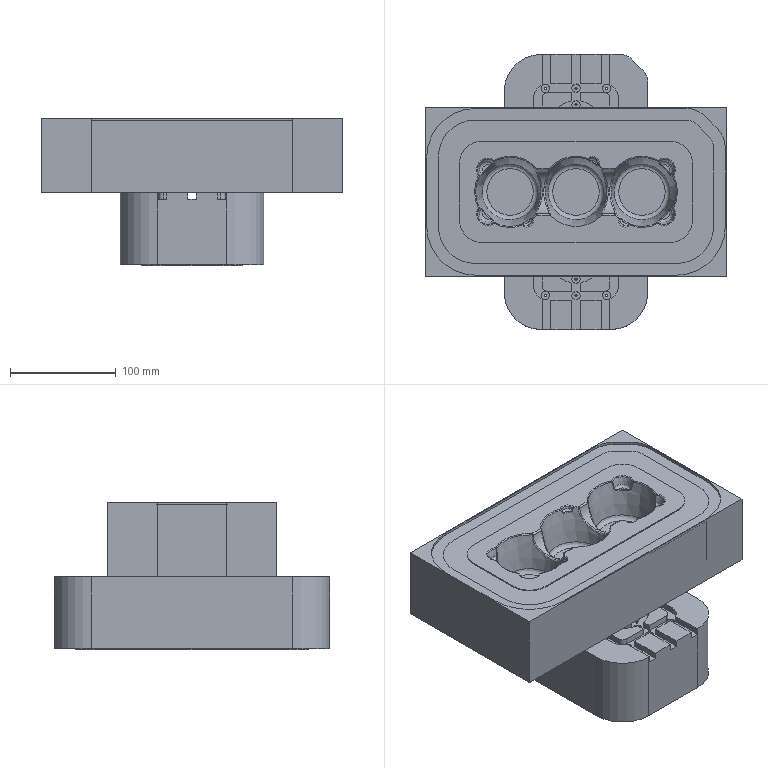NC program | NX | posted with a generic post | part box 284.317 x 260.317 x 139.5 mm
Lines 9197 to 10075 of 226982:
(B5 , TOOL : R2)
N18392 M6
N18394 G53
N18396 G17 G0 G90 X-90.649 Y-47.798 S8000 M3 M8
N18398 G43 Z220.5 H0
N18400 Z72.
N18402 G94 G1 Z69. F4500.
N18404 X-91.341 Y-47.76
N18406 X-91.498 Y-47.743
N18408 X-93.412 Y-47.435
N18410 X-93.627 Y-47.397
N18412 X-94.908 Y-47.053
N18414 X-95.487 Y-46.891
N18416 X-95.835 Y-46.78
N18418 X-96.947 Y-46.36
N18420 X-97.569 Y-46.118
N18422 X-97.691 Y-46.066
N18424 X-97.741 Y-46.044
N18426 X-99.64 Y-45.077
N18428 X-99.812 Y-44.976
N18430 X-101.411 Y-43.938
N18432 X-101.852 Y-43.595
N18434 G2 X-106.218 Y-39.132 R21.375
N18436 G1 X-107.256 Y-37.532
N18438 X-107.355 Y-37.364
N18440 X-108.237 Y-35.635
N18442 X-108.35 Y-35.412
N18444 X-108.398 Y-35.29
N18446 X-108.668 Y-34.596
N18448 X-109.06 Y-33.559
N18450 X-109.171 Y-33.213
N18452 X-109.333 Y-32.634
N18454 X-109.361 Y-32.521
N18456 X-109.549 Y-31.829
N18458 X-109.679 Y-31.342
N18460 X-109.715 Y-31.137
N18462 X-110.024 Y-29.218
N18464 X-110.039 Y-29.061
N18466 X-110.04 Y-29.04
N18468 X-110.079 Y-28.369
N18470 X-110.131 Y-27.331
N18472 X-110.142 Y-26.985
N18474 X-110.149 Y-26.654
N18476 Y26.971
N18478 X-110.131 Y27.328
N18480 X-110.079 Y28.369
N18482 X-110.04 Y29.04
N18484 X-110.024 Y29.218
N18486 X-109.829 Y30.445
N18488 X-109.716 Y31.131
N18490 X-109.679 Y31.342
N18492 X-109.456 Y32.173
N18494 X-109.172 Y33.207
N18496 G2 X-107.257 Y37.531 R21.069
N18498 G1 X-106.219 Y39.131
N18500 X-105.875 Y39.572
N18502 X-104.835 Y40.856
N18504 G2 X-99.812 Y44.975 R21.013
N18506 G1 X-99.645 Y45.074
N18508 X-97.812 Y46.013
N18510 X-97.569 Y46.114
N18512 X-96.876 Y46.387
N18514 X-95.839 Y46.779
N18516 X-95.493 Y46.89
N18518 X-94.914 Y47.052
N18520 X-93.628 Y47.397
N18522 X-93.417 Y47.434
N18524 X-91.497 Y47.743
N18526 X-91.341 Y47.757
N18528 X-90.649 Y47.798
N18530 X-89.265 Y47.868
N18532 X88.919
N18534 X89.265 Y47.861
N18536 X89.607 Y47.85
N18538 X90.649 Y47.798
N18540 X91.32 Y47.759
N18542 X91.498 Y47.743
N18544 X92.723 Y47.548
N18546 X93.627 Y47.397
N18548 X94.453 Y47.175
N18550 X95.487 Y46.891
N18552 G2 X99.812 Y44.976 R21.076
N18554 G1 X101.411 Y43.938
N18556 X101.852 Y43.595
N18558 X102.759 Y42.86
N18560 X103.136 Y42.554
N18562 X103.582 Y42.125 Z68.999
N18564 X104.618 Y41.083
N18566 X104.862 Y40.824 Z69.
N18568 X105.98 Y39.44
N18570 X106.218 Y39.132
N18572 X107.256 Y37.532
N18574 X107.355 Y37.364
N18576 X108.294 Y35.532
N18578 X108.395 Y35.289
N18580 X108.526 Y34.96
N18582 X109.06 Y33.559
N18584 X109.171 Y33.213
N18586 X109.333 Y32.634
N18588 X109.361 Y32.521
N18590 X109.456 Y32.175
N18592 X109.679 Y31.342
N18594 X109.715 Y31.137
N18596 X109.829 Y30.445
N18598 X110.024 Y29.218
N18600 X110.039 Y29.061
N18602 X110.079 Y28.369
N18604 X110.149 Y26.985
N18606 Y-26.639
N18608 X110.142 Y-26.985
N18610 X110.131 Y-27.328
N18612 X110.079 Y-28.369
N18614 X110.04 Y-29.04
N18616 X110.024 Y-29.218
N18618 X109.716 Y-31.131
N18620 X109.679 Y-31.342
N18622 X109.334 Y-32.628
N18624 X109.172 Y-33.207
N18626 X109.061 Y-33.554
N18628 X108.667 Y-34.597
N18630 X108.396 Y-35.286
N18632 X108.294 Y-35.532
N18634 X107.358 Y-37.359
N18636 X107.257 Y-37.531
N18638 X106.219 Y-39.131
N18640 X105.875 Y-39.572
N18642 X105.171 Y-40.442
N18644 X104.952 Y-40.713 Z68.998
N18646 X104.862 Y-40.824 Z69.
N18648 G2 X99.812 Y-44.975 R21.229
N18650 G1 X99.645 Y-45.074
N18652 X97.812 Y-46.013
N18654 X97.569 Y-46.114
N18656 X97.24 Y-46.245
N18658 X95.839 Y-46.779
N18660 X95.493 Y-46.89
N18662 X94.914 Y-47.052
N18664 X93.627 Y-47.397
N18666 X92.725 Y-47.548
N18668 X91.497 Y-47.743
N18670 X91.341 Y-47.757
N18672 X90.649 Y-47.798
N18674 X89.611 Y-47.85
N18676 X89.265 Y-47.861
N18678 X88.934 Y-47.868
N18680 X-89.251
N18682 X-89.607 Y-47.85
N18684 X-90.649 Y-47.798
N18686 Y-47.743
N18688 Y-47.512
N18690 X-91.373 Y-47.468
N18692 X-91.671 Y-47.427
N18694 X-93.071 Y-47.201
N18696 X-93.468 Y-47.136
N18698 X-93.757 Y-47.067
N18700 X-94.455 Y-46.879
N18702 G2 X-97.641 Y-45.775 R20.417
N18704 X-109.253 Y-31.829 R20.708
N18706 G1 X-109.346 Y-31.483
N18708 X-109.416 Y-31.187
N18710 X-109.708 Y-29.392
N18712 X-109.748 Y-29.093
N18714 X-109.751 Y-29.061
N18716 X-109.821 Y-27.82
N18718 X-109.854 Y-27.161
N18720 X-109.86 Y-26.985
N18722 X-109.863 Y26.801
N18724 X-109.846 Y27.331
N18726 G2 X-108.735 Y33.611 R20.049
N18728 G1 X-108.295 Y34.767
N18730 X-108.181 Y35.057
N18732 X-108.056 Y35.364
N18734 G2 X-102.685 Y42.554 R20.975
N18736 G1 X-102.524 Y42.684
N18738 X-101.721 Y43.334
N18740 X-101.316 Y43.651
N18742 G2 X-95.493 Y46.588 R20.765
N18744 G1 X-95.168 Y46.685
N18746 X-94.825 Y46.78
N18748 X-94.692 Y46.815
N18750 X-93.763 Y47.066
N18752 X-93.468 Y47.136
N18754 X-93.306 Y47.163
N18756 G2 X-88.919 Y47.583 R20.239
N18758 G1 X89.265 Y47.579
N18760 X91.084 Y47.487
N18762 X91.341 Y47.47
N18764 X91.373 Y47.467
N18766 X91.671 Y47.427
N18768 X93.468 Y47.135
N18770 X93.757 Y47.067
N18772 X94.801 Y46.786
N18774 G2 X104.835 Y40.405 R20.401
N18776 X107.107 Y37.215 R21.444
N18778 X108.754 Y33.559 R19.283
N18780 G1 X108.898 Y33.124
N18782 G2 X109.748 Y29.093 R20.718
N18784 G1 X109.751 Y29.061
N18786 X109.821 Y27.82
N18788 X109.854 Y27.161
N18790 X109.86 Y26.985
N18792 X109.863 Y-26.801
N18794 X109.846 Y-27.331
N18796 G2 X108.18 Y-35.057 R20.332
N18798 G1 X108.056 Y-35.364
N18800 G2 X105.615 Y-39.44 R19.949
N18802 G1 X104.835 Y-40.404
N18804 X104.773 Y-40.478
N18806 G2 X95.168 Y-46.685 R20.616
N18808 G1 X94.825 Y-46.78
N18810 X93.763 Y-47.066
N18812 X93.468 Y-47.135
N18814 X92.892 Y-47.231
N18816 G2 X89.435 Y-47.573 R18.487
N18818 G1 X88.919 Y-47.583
N18820 X-89.265 Y-47.579
N18822 X-90.649 Y-47.512
N18824 Y-47.226
N18826 G2 X-97.569 Y-45.49 R19.767
N18828 X-109.575 Y-26.985 R20.392
N18830 G1 X-109.578 Y26.74
N18832 X-109.575 Y26.985
N18834 G2 X-105.514 Y39.106 R20.649
N18836 X-93.238 Y46.884 R20.415
N18838 X-88.919 Y47.298 R20.666
N18840 G1 X89.265 Y47.294
N18842 X90.995 Y47.206
N18844 G2 X97.201 Y45.646 R19.84
N18846 X109.575 Y26.985 R20.388
N18848 G1 X109.578 Y-26.74
N18850 X109.575 Y-26.985
N18852 G2 X105.515 Y-39.106 R20.608
N18854 X88.919 Y-47.298 R20.491
N18856 G1 X-89.265 Y-47.294
N18858 X-90.649 Y-47.226
N18860 X-90.634 Y-46.942
N18862 X-91.198 Y-46.908
N18864 G2 X-96.877 Y-45.469 R20.309
N18866 G1 X-97.255 Y-45.322
N18868 G2 X-101.555 Y-42.735 R19.15
N18870 X-109.275 Y-27.331 R19.997
N18872 G1 X-109.292 Y-26.985
N18874 X-109.293 Y-26.946
N18876 X-109.29 Y27.028
N18878 G2 X-106.745 Y36.673 R19.973
N18880 X-89.265 Y47.01 R20.094
N18882 G1 X89.265
N18884 G2 X107.389 Y35.422 R20.108
N18886 G1 X107.456 Y35.289
N18888 G2 X109.293 Y26.946 R20.37
N18890 G1 X109.29 Y-27.028
N18892 G2 X106.745 Y-36.673 R19.973
N18894 X91.135 Y-46.912 R20.082
N18896 G1 X89.265 Y-47.01
N18898 X-89.265
N18900 X-90.634 Y-46.942
N18902 X-90.602 Y-46.658
N18904 G2 X-93.341 Y-46.284 R19.257
N18906 X-100.748 Y-43.004 R20.19
N18908 X-108.349 Y-31.898 R19.674
N18910 X-109.006 Y-27.009 R19.531
N18912 G1 X-109.008 Y26.961
N18914 G2 X-104.794 Y39.094 R19.862
N18916 X-89.268 Y46.726 R19.837
N18918 G1 X89.262
N18920 G2 X93.341 Y46.283 R20.044
N18922 X101.156 Y42.69 R19.954
N18924 X108.349 Y31.898 R19.619
N18926 X109.006 Y27.009 R19.487
N18928 G1 X109.008 Y-26.961
N18930 G2 X104.143 Y-39.895 R19.977
N18932 X89.268 Y-46.726 R19.927
N18934 G1 X-89.262
N18936 X-90.602 Y-46.658
N18938 X-90.587 Y-46.373
N18940 X-90.647 Y-46.37
N18942 X-90.987 Y-46.351
N18944 X-91.308 Y-46.326
N18946 G2 X-108.72 Y-26.985 R19.549
N18948 G1 X-108.722 Y26.904
N18950 G2 X-89.183 Y46.441 R19.568
N18952 G1 X89.265 Y46.439
N18954 G2 X108.602 Y29.061 R19.542
N18956 G1 X108.606 Y29.027
N18958 X108.631 Y28.715
N18960 X108.65 Y28.382
N18962 X108.72 Y26.985
N18964 X108.722 Y-26.904
N18966 X108.631 Y-28.715
N18968 X108.601 Y-29.061
N18970 X108.596 Y-29.106
N18972 G2 X89.183 Y-46.441 R19.566
N18974 G1 X-89.265 Y-46.439
N18976 X-90.587 Y-46.373
N18978 X-90.572 Y-46.088
N18980 X-91.043 Y-46.061
N18982 G2 X-108.434 Y-26.985 R19.275
N18984 G1 X-108.438 Y-21.936
N18986 X-108.437 Y26.843
N18988 G2 X-108.319 Y29.036 R44.188
N18990 X-94.344 Y45.432 R19.241
N18992 X-89.265 Y46.153 R18.273
N18994 G1 X-87.387 Y46.158
N18996 X89.062 Y46.157
N18998 X89.265 Y46.153
N19000 G2 X93.416 Y45.681 R18.878
N19002 X108.295 Y29.198 R19.259
N19004 G1 X108.311 Y29.084
N19006 X108.314 Y29.061
N19008 X108.341 Y28.767
N19010 X108.434 Y26.985
N19012 X108.438 Y21.936
N19014 X108.437 Y-26.843
N19016 G2 X108.319 Y-29.037 R43.992
N19018 X89.265 Y-46.153 R19.291
N19020 G1 X87.535 Y-46.158
N19022 X-89.062 Y-46.157
N19024 X-89.265 Y-46.153
N19026 X-89.4 Y-46.148
N19028 X-90.572 Y-46.088
N19030 X-90.557 Y-45.804
N19032 G2 X-108.153 Y-26.639 R18.972
N19034 G1 Y26.781
N19036 G2 X-89.265 Y45.868 R18.996
N19038 G1 X-87.531 Y45.873
N19040 X89.123 Y45.871
N19042 X89.265 Y45.868
N19044 G2 X108.153 Y26.639 R18.98
N19046 G1 Y-26.781
N19048 G2 X89.265 Y-45.868 R18.996
N19050 G1 X87.531 Y-45.873
N19052 X-89.123 Y-45.871
N19054 X-89.265 Y-45.868
N19056 X-89.458 Y-45.86
N19058 X-90.445 Y-45.81
N19060 X-90.557 Y-45.804
N19062 X-90.542 Y-45.519
N19064 G2 X-107.802 Y-28.223 R18.626
N19066 G1 X-107.866 Y-26.903
N19068 X-107.868 Y26.72
N19070 G2 X-89. Y45.587 R18.721
N19072 G1 X-88.919 Y45.588
N19074 X89.183 Y45.585
N19076 G2 X106.994 Y32.521 R18.729
N19078 X107.866 Y26.903 R18.927
N19080 G1 X107.868 Y-26.72
N19082 G2 X88.919 Y-45.588 R18.73
N19084 G1 X-89.183 Y-45.585
N19086 X-90.542 Y-45.519
N19088 X-90.527 Y-45.234
N19090 G2 X-107.494 Y-28.607 R18.362
N19092 G1 X-107.581 Y-26.964
N19094 X-107.583 Y26.639
N19096 G2 X-90.995 Y45.205 R18.433
N19098 G1 X-90.383 Y45.242
N19100 X-89.289 Y45.298
N19102 X-89.265 Y45.299
N19104 X89.265
N19106 G2 X106.446 Y33.213 R18.387
N19108 X107.581 Y26.964 R17.928
N19110 G1 X107.583 Y-26.639
N19112 G2 X89.265 Y-45.299 R18.435
N19114 G1 X-89.265
N19116 X-90.527 Y-45.234
N19118 X-90.513 Y-44.95
N19120 G2 X-107.294 Y-26.985 R18.091
N19122 G1 X-107.298 Y-18.573
N19124 X-107.294 Y26.985
N19126 G2 X-106.094 Y33.338 R18.163
N19128 X-89.265 Y45.014 R18.132
N19130 G1 X89.263
N19132 G2 X103.964 Y37.364 R18.152
N19134 X107.294 Y26.985 R18.404
N19136 G1 X107.298 Y18.573
N19138 X107.294 Y-26.985
N19140 G2 X106.305 Y-32.781 R18.457
N19142 X89.265 Y-45.014 R18.164
N19144 G1 X-89.263
N19146 X-90.513 Y-44.95
N19148 X-90.498 Y-44.665
N19150 G2 X-107.005 Y-27.08 R17.788
N19152 G1 X-107.008 Y-26.985
N19154 X-107.012 Y-26.741
N19156 X-107.013 Y-26.639
N19158 X-107.011 Y26.885
N19160 G2 X-89.165 Y44.73 R17.87
N19162 G1 X89.021 Y44.731
N19164 G2 X93.07 Y44.295 R19.93
N19166 X107.005 Y27.08 R17.829
N19168 G1 X107.008 Y26.985
N19170 X107.012 Y26.741
N19172 X107.013 Y26.639
N19174 X107.011 Y-26.885
N19176 G2 X89.165 Y-44.73 R17.87
N19178 G1 X-89.021 Y-44.731
N19180 X-89.265 Y-44.727
N19182 X-89.359 Y-44.724
N19184 X-89.611 Y-44.711
N19186 X-90.498 Y-44.665
N19188 X-90.482 Y-44.38
N19190 G2 X-106.716 Y-27.137 R17.508
N19192 G1 X-106.722 Y-26.985
N19194 X-106.728 Y-26.457
N19196 X-106.726 Y26.824
N19198 G2 X-104.664 Y35.113 R17.493
N19200 X-89.462 Y44.433 R17.525
N19202 G1 X-88.919 Y44.447
N19204 X89.081 Y44.445
N19206 G2 X103.176 Y37.466 R17.595
N19208 X106.722 Y26.985 R17.748
N19210 G1 X106.728 Y26.457
N19212 X106.726 Y-26.824
N19214 G2 X89.265 Y-44.441 R17.584
N19216 G1 X88.755 Y-44.447
N19218 X-89.081 Y-44.445
N19220 X-89.265 Y-44.441
N19222 X-89.417 Y-44.435
N19224 X-90.303 Y-44.39
N19226 X-90.482 Y-44.38
N19228 X-90.461 Y-44.095
N19230 G2 X-106.436 Y-26.985 R17.248
N19232 G1 X-106.443 Y-26.518
N19234 X-106.441 Y26.763
N19236 G2 X-88.919 Y44.162 R17.312
N19238 G1 X89.14 Y44.158
N19240 G2 X94.773 Y43.218 R17.668
N19242 X106.436 Y26.985 R17.273
N19244 G1 X106.443 Y26.518
N19246 X106.441 Y-26.763
N19248 G2 X88.919 Y-44.162 R17.312
N19250 G1 X-89.14 Y-44.158
N19252 X-89.803 Y-44.13
N19254 X-90.461 Y-44.095
N19256 X-90.446 Y-43.811
N19258 G2 X-106.154 Y-26.921 R16.957
N19260 G1 X-106.157 Y26.701
N19262 G2 X-88.634 Y43.877 R17.043
N19264 G1 X89.201 Y43.873
N19266 G2 X105.941 Y29.482 R16.96
N19268 G1 X106.032 Y28.875
N19270 X106.05 Y28.715
N19272 X106.065 Y28.562
N19274 X106.099 Y28.023
N19276 X106.154 Y26.921
N19278 X106.157 Y-26.701
N19280 G2 X88.634 Y-43.877 R17.042
N19282 G1 X-89.201 Y-43.873
N19284 X-90.446 Y-43.811
N19286 X-90.431 Y-43.526
N19288 G2 X-105.424 Y-30.689 R16.629
N19290 X-105.873 Y-26.64 R17.53
N19292 G1 X-105.872 Y26.639
N19294 G2 X-90.649 Y43.514 R16.731
N19296 G1 X-90.365 Y43.53
N19298 X-89.27 Y43.587
N19300 X-88.985 Y43.592
N19302 X-88.919
N19304 X88.919
N19306 G2 X104.143 Y34.256 R16.721
N19308 X105.814 Y28.023 R16.056
N19310 G1 X105.868 Y26.985
N19312 X105.873 Y26.64
N19314 X105.872 Y-26.639
N19316 G2 X90.649 Y-43.514 R16.729
N19318 G1 X90.365 Y-43.53
N19320 X89.27 Y-43.587
N19322 X88.985 Y-43.592
N19324 X88.919
N19326 X-88.919
N19328 X-89.261 Y-43.587
N19330 X-90.431 Y-43.526
N19332 X-90.415 Y-43.241
N19334 X-90.633 Y-43.229
N19336 G2 X-105.587 Y-26.701 R16.403
N19338 G1 X-105.588 Y-26.355
N19340 X-105.587 Y26.579
N19342 G2 X-88.858 Y43.307 R16.464
N19344 G1 X88.919
N19346 G2 X92.764 Y42.9 R17.06
N19348 X105.587 Y26.701 R16.405
N19350 G1 X105.588 Y26.355
N19352 X105.587 Y-26.579
N19354 G2 X88.858 Y-43.307 R16.467
N19356 G1 X-88.919
N19358 X-89.264 Y-43.302
N19360 X-89.955 Y-43.266
N19362 X-90.415 Y-43.241
N19364 X-90.4 Y-42.956
N19366 G2 X-104.489 Y-31.921 R16.067
N19368 X-105.303 Y-26.416 R17.107
N19370 G1 X-105.299 Y26.867
N19372 G2 X-89.147 Y43.018 R16.167
N19374 G1 X-83.254 Y43.022
N19376 X89.039 Y43.02
N19378 G2 X95.955 Y41.516 R16.73
N19380 X105.296 Y26.985 R16.104
N19382 G1 X105.303 Y26.416
N19384 X105.299 Y-26.867
N19386 G2 X89.147 Y-43.018 R16.166
N19388 G1 X83.254 Y-43.022
N19390 X-89.039 Y-43.02
N19392 X-89.265 Y-43.015
N19394 X-89.376 Y-43.01
N19396 X-90.303 Y-42.962
N19398 X-90.4 Y-42.956
N19400 X-90.384 Y-42.671
N19402 G2 X-105.002 Y-27.153 R15.804
N19404 G1 X-105.016 Y-26.639
N19406 Y26.639
N19408 G2 X-104.857 Y29.039 R17.293
N19410 X-89.265 Y42.728 R15.86
N19412 G1 X-88.573 Y42.737
N19414 X88.919 Y42.735
N19416 G2 X104.894 Y28.782 R15.849
N19418 X105.016 Y26.639 R20.313
N19420 G1 Y-26.639
N19422 G2 X103.797 Y-32.949 R16.109
N19424 X89.265 Y-42.728 R15.869
N19426 G1 X88.573 Y-42.737
N19428 X-88.919 Y-42.735
N19430 X-89.432 Y-42.721
N19432 X-90.384 Y-42.671
N19434 X-90.366 Y-42.386
N19436 G2 X-104.68 Y-27.869 R15.479
N19438 G1 X-104.728 Y-26.879
N19440 X-104.733 Y-26.293
N19442 X-104.73 Y26.744
N19444 G2 X-103.374 Y33.213 R15.519
N19446 X-89.265 Y42.443 R15.572
N19448 G1 X-88.675 Y42.452
N19450 X88.919 Y42.45
N19452 G2 X102.477 Y34.943 R15.627
N19454 X104.732 Y26.639 R15.801
N19456 G1 X104.73 Y-26.744
N19458 G2 X102.973 Y-34.037 R15.504
N19460 X89.265 Y-42.443 R15.567
N19462 G1 X88.675 Y-42.452
N19464 X-88.919 Y-42.45
N19466 X-89.49 Y-42.433
N19468 X-90.366 Y-42.386
N19470 X-90.35 Y-42.102
N19472 G2 X-104.372 Y-28.253 R15.215
N19474 G1 X-104.442 Y-26.939
N19476 X-104.448 Y-26.599
N19478 X-104.446 Y26.682
N19480 G2 X-88.614 Y42.167 R15.345
N19482 G1 X88.878
N19484 G2 X100.478 Y37.161 R15.381
N19486 X104.448 Y26.599 R15.432
N19488 G1 X104.446 Y-26.682
N19490 G2 X88.614 Y-42.167 R15.345
N19492 G1 X-88.878
N19494 X-89.218 Y-42.161
N19496 X-89.265 Y-42.159
N19498 X-90.35 Y-42.102
N19500 X-90.332 Y-41.818
N19502 G2 X-104.155 Y-27.001 R14.971
N19504 G1 X-104.163 Y-26.639
N19506 X-104.162 Y26.618
N19508 G2 X-92.361 Y41.534 R15.058
N19510 X-88.922 Y41.882 R16.461
N19512 G1 X88.916
N19514 G2 X102.861 Y32.981 R15.014
N19516 X104.163 Y26.639 R15.632
N19518 G1 X104.162 Y-26.618
N19520 G2 X90.649 Y-41.798 R15.04
N19522 G1 X90.348 Y-41.818
N19524 X89.267 Y-41.875
N19526 X88.922 Y-41.882
N19528 X-88.916
N19530 X-89.263 Y-41.875
N19532 X-90.263 Y-41.822
N19534 X-90.332 Y-41.818
N19536 X-90.301 Y-41.534
N19538 G2 X-103.869 Y-26.985 R14.664
N19540 G1 X-103.878 Y-26.375
N19542 X-103.876 Y26.639
N19544 G2 X-92.293 Y41.256 R14.773
N19546 X-88.838 Y41.597 R16.102
N19548 G1 X88.998 Y41.595
N19550 G2 X101.825 Y34.371 R14.776
N19552 X103.878 Y26.375 R15.062
N19554 G1 X103.876 Y-26.639
N19556 G2 X88.838 Y-41.597 R14.77
N19558 G1 X-88.998 Y-41.595
N19560 X-89.265 Y-41.589
N19562 X-89.314 Y-41.587
N19564 X-90.301 Y-41.534
N19566 X-90.285 Y-41.249
N19568 G2 X-103.582 Y-26.985 R14.379
N19570 G1 X-103.593 Y-26.293
N19572 X-103.59 Y26.639
N19574 G2 X-89.265 Y41.301 R14.466
N19576 G1 X-88.573 Y41.312
N19578 X88.919 Y41.31
N19580 G2 X94.556 Y40.249 R14.802
N19582 X103.582 Y26.985 R14.365
N19584 G1 X103.593 Y26.293
N19586 X103.59 Y-26.639
N19588 G2 X89.265 Y-41.301 R14.466
N19590 G1 X88.573 Y-41.312
N19592 X-88.919 Y-41.31
N19594 X-89.611 Y-41.285
N19596 X-89.957 Y-41.267
N19598 X-90.285 Y-41.249
N19600 X-90.268 Y-40.963
N19602 G2 X-103.016 Y-29.665 R14.057
N19604 X-103.308 Y-26.293 R15.915
N19606 G1 X-103.305 Y26.639
N19608 G2 X-89.265 Y41.016 R14.18
N19610 G1 X-88.573 Y41.027
N19612 X88.919 Y41.025
N19614 G2 X100.438 Y35.411 R14.202
N19616 X103.302 Y26.837 R14.342
N19618 G1 X103.308 Y26.293
N19620 X103.305 Y-26.639
N19622 G2 X89.265 Y-41.016 R14.177
N19624 G1 X88.573 Y-41.027
N19626 X-88.919 Y-41.025
N19628 X-89.611 Y-41.
N19630 X-90.106 Y-40.973
N19632 X-90.268 Y-40.963
N19634 X-90.25 Y-40.679
N19636 G2 X-103.001 Y-27.228 R13.799
N19638 G1 X-103.021 Y-26.639
N19640 X-103.02 Y26.725
N19642 G2 X-101.952 Y32.175 R13.917
N19644 X-89.265 Y40.732 R13.879
N19646 G1 X-88.655 Y40.742
N19648 X88.919 Y40.74
N19650 G2 X93.622 Y39.991 R14.393
N19652 X103.016 Y26.897 R13.825
N19654 G1 X103.021 Y26.639
N19656 X103.022 Y26.557
N19658 X103.02 Y-26.725
N19660 G2 X102.413 Y-30.899 R14.116
N19662 X89.265 Y-40.732 R13.881
N19664 G1 X88.655 Y-40.742
N19666 X-88.919 Y-40.74
N19668 X-89.507 Y-40.72
N19670 X-90.164 Y-40.685
N19672 X-90.25 Y-40.679
N19674 X-90.221 Y-40.396
N19676 G2 X-102.73 Y-26.956 R13.526
N19678 G1 X-102.738 Y-26.618
N19680 X-102.736 Y26.639
N19682 G2 X-92.017 Y40.148 R13.641
N19684 X-88.941 Y40.456 R15.94
N19686 G1 X88.897
N19688 G2 X97.25 Y37.78 R13.882
N19690 X102.73 Y26.956 R13.625
N19692 G1 X102.738 Y26.618
N19694 X102.736 Y-26.639
N19696 G2 X90.395 Y-40.386 R13.617
N19698 G1 X90.303 Y-40.392
N19700 X89.265 Y-40.447
N19702 X88.941 Y-40.456
N19704 X-88.897
N19706 X-89.236 Y-40.449
N19708 X-89.265 Y-40.447
N19710 X-90.221 Y-40.396
N19712 X-90.205 Y-40.111
N19714 G2 X-102.442 Y-27.015 R13.268
N19716 G1 X-102.451 Y-26.682
N19718 X-102.452 Y-26.639
N19720 X-102.451 Y26.598
N19722 G2 X-101.74 Y31.133 R13.818
N19724 X-88.922 Y40.172 R13.343
N19726 G1 X88.917 Y40.171
N19728 G2 X99.064 Y35.746 R13.411
N19730 X102.442 Y27.015 R13.445
N19732 G1 X102.451 Y26.682
N19734 X102.452 Y26.639
N19736 X102.451 Y-26.598
N19738 G2 X101.741 Y-31.132 R13.847
N19740 X88.922 Y-40.172 R13.345
N19742 G1 X-88.917 Y-40.171
N19744 X-89.265 Y-40.162
N19746 X-90.205 Y-40.111
N19748 X-90.189 Y-39.826
N19750 G2 X-102.156 Y-26.985 R12.954
N19752 G1 X-102.167 Y-26.293
N19754 X-102.164 Y26.639
N19756 G2 X-100.855 Y32.521 R13.043
N19758 X-89.173 Y39.879 R13.019
N19760 G1 X-88.573 Y39.887
N19762 X89.016 Y39.883
N19764 G2 X94.455 Y38.75 R13.358
N19766 X102.156 Y26.985 R12.974
N19768 G1 X102.167 Y26.293
N19770 X102.164 Y-26.639
N19772 G2 X101.023 Y-32.175 R13.368
N19774 X89.173 Y-39.879 R13.045
N19776 G1 X88.573 Y-39.887
N19778 X-89.016 Y-39.883
N19780 X-89.611 Y-39.858
N19782 X-89.956 Y-39.839
N19784 X-90.189 Y-39.826
N19786 X-90.17 Y-39.54
N19788 G2 X-101.87 Y-26.985 R12.661
N19790 G1 X-101.882 Y-26.293
N19792 X-101.879 Y26.639
N19794 G2 X-89.11 Y39.595 R12.772
N19796 G1 X-88.573 Y39.602
N19798 X88.919 Y39.599
N19800 G2 X100.706 Y32.198 R12.757
N19802 X101.87 Y26.985 R12.922
N19804 G1 X101.882 Y26.293
N19806 X101.879 Y-26.639
N19808 G2 X89.11 Y-39.595 R12.772
N19810 G1 X88.573 Y-39.602
N19812 X-88.919 Y-39.599
N19814 X-89.408 Y-39.583
N19816 X-90.17 Y-39.54
N19818 X-90.121 Y-39.258
N19820 G2 X-101.591 Y-26.856 R12.401
N19822 G1 X-101.596 Y-26.639
N19824 X-101.597 Y-26.516
N19826 X-101.595 Y26.639
N19828 G2 X-90.303 Y39.247 R12.477
N19830 G1 X-90.139 Y39.259
N19832 X-89.047 Y39.313
N19834 X-83.15 Y39.316
N19836 X88.919 Y39.315
N19838 G2 X95.619 Y37.498 R12.759
N19840 X101.596 Y26.639 R12.494
N19842 G1 X101.597 Y26.516
N19844 X101.595 Y-26.639
N19846 G2 X90.303 Y-39.247 R12.475
N19848 G1 X90.138 Y-39.259
N19850 X89.047 Y-39.313
N19852 X83.15 Y-39.316
N19854 X-88.919 Y-39.315
N19856 X-89.466 Y-39.295
N19858 X-89.794 Y-39.277
N19860 X-90.121 Y-39.258
N19862 X-90.104 Y-38.974
N19864 G2 X-101.304 Y-26.915 R12.123
N19866 G1 X-101.311 Y-26.639
N19868 X-101.312 Y-26.577
N19870 X-101.309 Y26.705
N19872 G2 X-100.153 Y32.013 R12.39
N19874 X-90.303 Y38.961 R12.172
N19876 X-88.919 Y39.03 R28.075
N19878 G1 X88.919
N19880 G2 X93.302 Y38.287 R12.711
N19882 X101.304 Y26.915 R12.121
N19884 G1 X101.311 Y26.639
N19886 X101.312 Y26.577
N19888 X101.309 Y-26.705
N19890 G2 X100.421 Y-31.398 R12.52
N19892 X90.303 Y-38.961 R12.184
N19894 X88.919 Y-39.03 R28.235
N19896 G1 X-88.919
N19898 X-89.523 Y-39.007
N19900 X-89.852 Y-38.989
N19902 X-90.104 Y-38.974
N19904 X-90.086 Y-38.689
N19906 G2 X-101.016 Y-26.985 R11.816
N19908 G1 X-101.027 Y-26.639
N19910 X-101.026 Y26.639
N19912 G2 X-100.462 Y30.445 R12.478
N19914 X-90.303 Y38.676 R11.909
N19916 G1 X-90.01 Y38.695
N19918 X-89.279 Y38.734
N19920 X-88.921 Y38.746
N19922 X88.917
N19924 G2 X100.085 Y31.483 R11.907
N19926 X101.027 Y26.639 R12.303
N19928 G1 X101.026 Y-26.639
N19930 G2 X90.303 Y-38.676 R11.922
N19932 G1 X90.01 Y-38.695
N19934 X89.279 Y-38.735
N19936 X88.921 Y-38.746
N19938 X-88.917
N19940 X-89.253 Y-38.736
N19942 X-89.909 Y-38.7
N19944 X-90.086 Y-38.689
N19946 X-90.069 Y-38.405
N19948 G2 X-100.728 Y-27.035 R11.529
N19950 G1 X-100.74 Y-26.699
N19952 X-100.741 Y26.581
N19954 G2 X-88.92 Y38.461 R11.662
N19956 G1 X88.919
N19958 G2 X99.731 Y31.586 R11.633
N19960 X100.74 Y26.699 R11.981
N19962 G1 X100.741 Y-26.581
N19964 G2 X88.92 Y-38.461 R11.662
N19966 G1 X-88.919
N19968 X-89.263 Y-38.45
N19970 X-89.956 Y-38.412
N19972 X-90.069 Y-38.405
N19974 X-90.048 Y-38.12
N19976 G2 X-100.403 Y-27.746 R11.23
N19978 G1 X-100.452 Y-26.755
N19980 X-100.456 Y-24.82
N19982 X-100.455 Y26.521
N19984 G2 X-89.154 Y38.168 R11.363
N19986 G1 X-88.573 Y38.176
N19988 X88.919 Y38.173
N19990 G2 X93.141 Y37.434 R11.733
N19992 X100.422 Y27.416 R11.232
N19994 G1 X100.452 Y26.755
N19996 X100.456 Y24.82
N19998 X100.455 Y-26.521
N20000 G2 X89.154 Y-38.168 R11.364
N20002 G1 X88.573 Y-38.176
N20004 X-88.919 Y-38.173
N20006 X-89.611 Y-38.145
N20008 X-89.986 Y-38.124
N20010 X-90.048 Y-38.12
N20012 X-90.029 Y-37.835
N20014 G2 X-100.133 Y-27.474 R10.933
N20016 G1 X-100.165 Y-26.814
N20018 X-100.172 Y-26.293
N20020 X-100.171 Y26.46
N20022 G2 X-99.773 Y29.753 R11.862
N20024 X-88.919 Y37.888 R11.073
N20026 G1 X-88.739 Y37.891
N20028 X88.919 Y37.888
N20030 G2 X97.282 Y34.31 R11.155
N20032 X100.165 Y26.814 R11.121
N20034 G1 X100.172 Y26.293
N20036 X100.171 Y-26.46
N20038 G2 X99.773 Y-29.753 R12.007
N20040 X88.919 Y-37.888 R11.075
N20042 G1 X88.739 Y-37.891
N20044 X-88.919 Y-37.888
N20046 X-89.425 Y-37.87
N20048 X-90.029 Y-37.835
N20050 X-90.008 Y-37.55
N20052 G2 X-99.878 Y-26.873 R10.692
N20054 G1 X-99.886 Y-26.293
N20056 Y26.399
N20058 G2 X-99.123 Y30.791 R11.171
N20060 X-88.919 Y37.604 R10.778
N20062 G1 X88.919 Y37.603
N20064 G2 X94.592 Y36.118 R11.051
N20066 X99.878 Y26.873 R10.755
N20068 G1 X99.886 Y26.293
N20070 Y-26.399
N20072 G2 X99.124 Y-30.791 R11.362
N20074 X89.028 Y-37.601 R10.773
N20076 G1 X85.935 Y-37.606
N20078 X-88.919 Y-37.603
N20080 X-89.482 Y-37.581
N20082 X-90.008 Y-37.55
N20084 X-89.957 Y-37.268
N20086 G2 X-99.57 Y-27.331 R10.376
N20088 G1 X-99.6 Y-26.639
N20090 X-99.599 Y26.639
N20092 G2 X-99.073 Y30.099 R10.792
N20094 X-88.965 Y37.319 R10.503
N20096 G1 X-88.919 Y37.32
N20098 X88.919 Y37.319
N20100 G2 X92.725 Y36.675 R11.083
N20102 X99.57 Y27.331 R10.365
N20104 G1 X99.6 Y26.639
N20106 Y-26.639
N20108 G2 X99.074 Y-30.099 R10.915
N20110 X88.965 Y-37.319 R10.505
N20112 G1 X88.919 Y-37.32
N20114 X-88.919 Y-37.319
N20116 X-89.539 Y-37.293
N20118 X-89.867 Y-37.274
N20120 X-89.957 Y-37.268
N20122 X-89.924 Y-36.985
N20124 G2 X-99.303 Y-26.991 R10.116
N20126 G1 X-99.315 Y-26.659
N20128 Y26.621
N20130 G2 X-98.771 Y30.099 R10.713
N20132 X-89.266 Y37.023 R10.192
N20134 G1 X-88.922 Y37.035
N20136 X88.917
N20138 G2 X95.199 Y35.036 R10.437
N20140 X99.303 Y26.991 R10.182
N20142 G1 X99.315 Y26.659